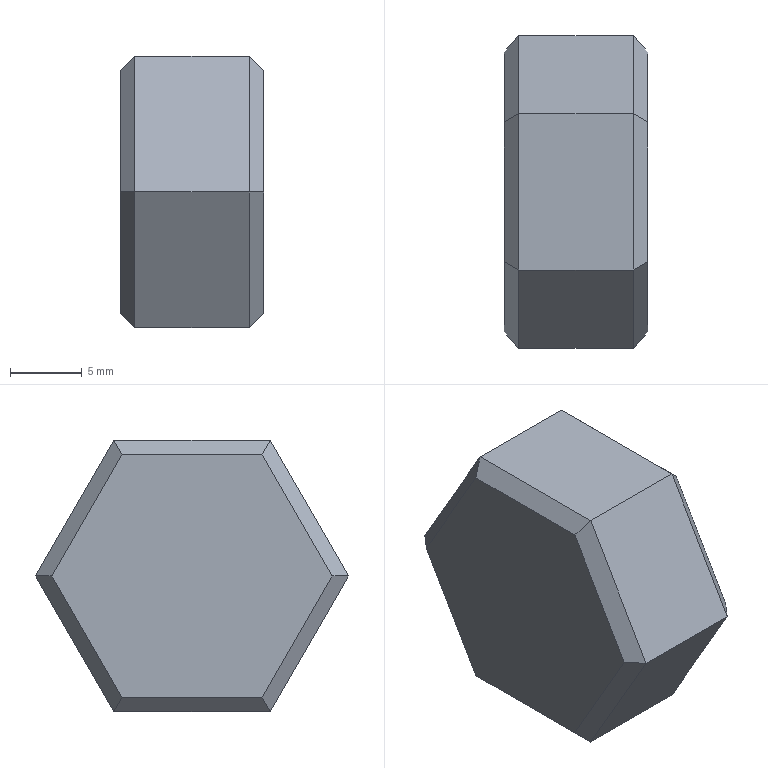Part | STEP file | Tube feed_id798_x_t | 1 solid | 20 faces | box 10 x 21.824 x 18.9 mm | volume 3030 mm3 | plane 20
STEP:
#1=CARTESIAN_POINT('',(0.,0.,0.));
#2=DIRECTION('',(0.,0.,1.));
#3=DIRECTION('',(1.,0.,0.));
#4=AXIS2_PLACEMENT_3D('',#1,#2,#3);
#5=CARTESIAN_POINT('',(413.,4.58,-40.45));
#6=VERTEX_POINT('',#5);
#7=CARTESIAN_POINT('',(421.,4.58,-40.45));
#8=VERTEX_POINT('',#7);
#9=CARTESIAN_POINT('',(412.,4.58,-40.45));
#10=DIRECTION('',(1.,0.,0.));
#11=VECTOR('',#10,1.);
#12=LINE('',#9,#11);
#13=CARTESIAN_POINT('',(412.,4.58,-40.45));
#14=DIRECTION('',(0.,0.866,0.5));
#15=DIRECTION('',(0.,-0.5,0.866));
#16=AXIS2_PLACEMENT_3D('',#13,#14,#15);
#17=PLANE('',#16);
#18=CARTESIAN_POINT('',(0.,0.));
#19=DIRECTION('',(0.,1.));
#20=VECTOR('',#19,1.);
#21=LINE('',#18,#20);
#22=(GEOMETRIC_REPRESENTATION_CONTEXT(2)PARAMETRIC_REPRESENTATION_CONTEXT()REPRESENTATION_CONTEXT('',''));
#23=DEFINITIONAL_REPRESENTATION('',(#21),#22);
#24=PCURVE('',#17,#23);
#25=CARTESIAN_POINT('',(412.,15.492,-40.45));
#26=DIRECTION('',(0.,0.,1.));
#27=DIRECTION('',(0.,-1.,0.));
#28=AXIS2_PLACEMENT_3D('',#25,#26,#27);
#29=PLANE('',#28);
#30=CARTESIAN_POINT('',(10.912,0.));
#31=DIRECTION('',(0.,1.));
#32=VECTOR('',#31,1.);
#33=LINE('',#30,#32);
#34=(GEOMETRIC_REPRESENTATION_CONTEXT(2)PARAMETRIC_REPRESENTATION_CONTEXT()REPRESENTATION_CONTEXT('',''));
#35=DEFINITIONAL_REPRESENTATION('',(#33),#34);
#36=PCURVE('',#29,#35);
#37=SURFACE_CURVE('',#12,(#24,#36),.PCURVE_S1.);
#38=EDGE_CURVE('',#6,#8,#37,.T.);
#39=ORIENTED_EDGE('',*,*,#38,.T.);
#40=CARTESIAN_POINT('',(421.,-0.8763,-31.));
#41=VERTEX_POINT('',#40);
#42=CARTESIAN_POINT('',(421.,4.58,-40.45));
#43=DIRECTION('',(0.,-0.5,0.866));
#44=VECTOR('',#43,1.);
#45=LINE('',#42,#44);
#46=CARTESIAN_POINT('',(0.,9.));
#47=DIRECTION('',(1.,0.));
#48=VECTOR('',#47,1.);
#49=LINE('',#46,#48);
#50=(GEOMETRIC_REPRESENTATION_CONTEXT(2)PARAMETRIC_REPRESENTATION_CONTEXT()REPRESENTATION_CONTEXT('',''));
#51=DEFINITIONAL_REPRESENTATION('',(#49),#50);
#52=PCURVE('',#17,#51);
#53=CARTESIAN_POINT('',(421.,4.58,-40.45));
#54=DIRECTION('',(-0.7071,0.6124,0.3536));
#55=DIRECTION('',(0.,-0.5,0.866));
#56=AXIS2_PLACEMENT_3D('',#53,#54,#55);
#57=PLANE('',#56);
#58=CARTESIAN_POINT('',(0.,0.));
#59=DIRECTION('',(1.,0.));
#60=VECTOR('',#59,1.);
#61=LINE('',#58,#60);
#62=(GEOMETRIC_REPRESENTATION_CONTEXT(2)PARAMETRIC_REPRESENTATION_CONTEXT()REPRESENTATION_CONTEXT('',''));
#63=DEFINITIONAL_REPRESENTATION('',(#61),#62);
#64=PCURVE('',#57,#63);
#65=SURFACE_CURVE('',#45,(#52,#64),.PCURVE_S1.);
#66=EDGE_CURVE('',#8,#41,#65,.T.);
#67=ORIENTED_EDGE('',*,*,#66,.T.);
#68=CARTESIAN_POINT('',(413.,-0.8763,-31.));
#69=VERTEX_POINT('',#68);
#70=CARTESIAN_POINT('',(412.,-0.8763,-31.));
#71=DIRECTION('',(1.,0.,0.));
#72=VECTOR('',#71,1.);
#73=LINE('',#70,#72);
#74=CARTESIAN_POINT('',(10.912,0.));
#75=DIRECTION('',(0.,1.));
#76=VECTOR('',#75,1.);
#77=LINE('',#74,#76);
#78=(GEOMETRIC_REPRESENTATION_CONTEXT(2)PARAMETRIC_REPRESENTATION_CONTEXT()REPRESENTATION_CONTEXT('',''));
#79=DEFINITIONAL_REPRESENTATION('',(#77),#78);
#80=PCURVE('',#17,#79);
#81=CARTESIAN_POINT('',(412.,-0.8763,-31.));
#82=DIRECTION('',(0.,0.866,-0.5));
#83=DIRECTION('',(0.,0.5,0.866));
#84=AXIS2_PLACEMENT_3D('',#81,#82,#83);
#85=PLANE('',#84);
#86=CARTESIAN_POINT('',(0.,0.));
#87=DIRECTION('',(0.,1.));
#88=VECTOR('',#87,1.);
#89=LINE('',#86,#88);
#90=(GEOMETRIC_REPRESENTATION_CONTEXT(2)PARAMETRIC_REPRESENTATION_CONTEXT()REPRESENTATION_CONTEXT('',''));
#91=DEFINITIONAL_REPRESENTATION('',(#89),#90);
#92=PCURVE('',#85,#91);
#93=SURFACE_CURVE('',#73,(#80,#92),.PCURVE_S1.);
#94=EDGE_CURVE('',#69,#41,#93,.T.);
#95=ORIENTED_EDGE('',*,*,#94,.F.);
#96=CARTESIAN_POINT('',(413.,4.58,-40.45));
#97=DIRECTION('',(0.,0.5,-0.866));
#98=VECTOR('',#97,1.);
#99=LINE('',#96,#98);
#100=CARTESIAN_POINT('',(0.,1.));
#101=DIRECTION('',(-1.,0.));
#102=VECTOR('',#101,1.);
#103=LINE('',#100,#102);
#104=(GEOMETRIC_REPRESENTATION_CONTEXT(2)PARAMETRIC_REPRESENTATION_CONTEXT()REPRESENTATION_CONTEXT('',''));
#105=DEFINITIONAL_REPRESENTATION('',(#103),#104);
#106=PCURVE('',#17,#105);
#107=CARTESIAN_POINT('',(412.,-13.215,-7.629));
#108=DIRECTION('',(-0.7071,-0.6124,-0.3536));
#109=DIRECTION('',(0.,0.5,-0.866));
#110=AXIS2_PLACEMENT_3D('',#107,#108,#109);
#111=PLANE('',#110);
#112=CARTESIAN_POINT('',(37.321,1.414));
#113=DIRECTION('',(1.,0.));
#114=VECTOR('',#113,1.);
#115=LINE('',#112,#114);
#116=(GEOMETRIC_REPRESENTATION_CONTEXT(2)PARAMETRIC_REPRESENTATION_CONTEXT()REPRESENTATION_CONTEXT('',''));
#117=DEFINITIONAL_REPRESENTATION('',(#115),#116);
#118=PCURVE('',#111,#117);
#119=SURFACE_CURVE('',#99,(#106,#118),.PCURVE_S1.);
#120=EDGE_CURVE('',#69,#6,#119,.T.);
#121=ORIENTED_EDGE('',*,*,#120,.T.);
#122=EDGE_LOOP('',(#39,#67,#95,#121));
#123=FACE_BOUND('',#122,.T.);
#124=ADVANCED_FACE('',(#123),#17,.F.);
#125=ORIENTED_EDGE('',*,*,#94,.T.);
#126=CARTESIAN_POINT('',(421.,4.58,-21.55));
#127=VERTEX_POINT('',#126);
#128=CARTESIAN_POINT('',(421.,-0.8763,-31.));
#129=DIRECTION('',(0.,0.5,0.866));
#130=VECTOR('',#129,1.);
#131=LINE('',#128,#130);
#132=CARTESIAN_POINT('',(0.,9.));
#133=DIRECTION('',(1.,0.));
#134=VECTOR('',#133,1.);
#135=LINE('',#132,#134);
#136=(GEOMETRIC_REPRESENTATION_CONTEXT(2)PARAMETRIC_REPRESENTATION_CONTEXT()REPRESENTATION_CONTEXT('',''));
#137=DEFINITIONAL_REPRESENTATION('',(#135),#136);
#138=PCURVE('',#85,#137);
#139=CARTESIAN_POINT('',(421.,-0.8763,-31.));
#140=DIRECTION('',(-0.7071,0.6124,-0.3536));
#141=DIRECTION('',(0.,0.5,0.866));
#142=AXIS2_PLACEMENT_3D('',#139,#140,#141);
#143=PLANE('',#142);
#144=CARTESIAN_POINT('',(0.,0.));
#145=DIRECTION('',(1.,0.));
#146=VECTOR('',#145,1.);
#147=LINE('',#144,#146);
#148=(GEOMETRIC_REPRESENTATION_CONTEXT(2)PARAMETRIC_REPRESENTATION_CONTEXT()REPRESENTATION_CONTEXT('',''));
#149=DEFINITIONAL_REPRESENTATION('',(#147),#148);
#150=PCURVE('',#143,#149);
#151=SURFACE_CURVE('',#131,(#138,#150),.PCURVE_S1.);
#152=EDGE_CURVE('',#41,#127,#151,.T.);
#153=ORIENTED_EDGE('',*,*,#152,.T.);
#154=CARTESIAN_POINT('',(413.,4.58,-21.55));
#155=VERTEX_POINT('',#154);
#156=CARTESIAN_POINT('',(412.,4.58,-21.55));
#157=DIRECTION('',(1.,0.,0.));
#158=VECTOR('',#157,1.);
#159=LINE('',#156,#158);
#160=CARTESIAN_POINT('',(10.912,0.));
#161=DIRECTION('',(0.,1.));
#162=VECTOR('',#161,1.);
#163=LINE('',#160,#162);
#164=(GEOMETRIC_REPRESENTATION_CONTEXT(2)PARAMETRIC_REPRESENTATION_CONTEXT()REPRESENTATION_CONTEXT('',''));
#165=DEFINITIONAL_REPRESENTATION('',(#163),#164);
#166=PCURVE('',#85,#165);
#167=CARTESIAN_POINT('',(412.,4.58,-21.55));
#168=DIRECTION('',(0.,0.,-1.));
#169=DIRECTION('',(-1.,0.,0.));
#170=AXIS2_PLACEMENT_3D('',#167,#168,#169);
#171=PLANE('',#170);
#172=CARTESIAN_POINT('',(0.,0.));
#173=DIRECTION('',(-1.,0.));
#174=VECTOR('',#173,1.);
#175=LINE('',#172,#174);
#176=(GEOMETRIC_REPRESENTATION_CONTEXT(2)PARAMETRIC_REPRESENTATION_CONTEXT()REPRESENTATION_CONTEXT('',''));
#177=DEFINITIONAL_REPRESENTATION('',(#175),#176);
#178=PCURVE('',#171,#177);
#179=SURFACE_CURVE('',#159,(#166,#178),.PCURVE_S1.);
#180=EDGE_CURVE('',#155,#127,#179,.T.);
#181=ORIENTED_EDGE('',*,*,#180,.F.);
#182=CARTESIAN_POINT('',(413.,-0.8763,-31.));
#183=DIRECTION('',(0.,-0.5,-0.866));
#184=VECTOR('',#183,1.);
#185=LINE('',#182,#184);
#186=CARTESIAN_POINT('',(0.,1.));
#187=DIRECTION('',(-1.,0.));
#188=VECTOR('',#187,1.);
#189=LINE('',#186,#188);
#190=(GEOMETRIC_REPRESENTATION_CONTEXT(2)PARAMETRIC_REPRESENTATION_CONTEXT()REPRESENTATION_CONTEXT('',''));
#191=DEFINITIONAL_REPRESENTATION('',(#189),#190);
#192=PCURVE('',#85,#191);
#193=CARTESIAN_POINT('',(412.,13.632,-7.871));
#194=DIRECTION('',(-0.7071,-0.6124,0.3536));
#195=DIRECTION('',(0.,-0.5,-0.866));
#196=AXIS2_PLACEMENT_3D('',#193,#194,#195);
#197=PLANE('',#196);
#198=CARTESIAN_POINT('',(27.285,1.414));
#199=DIRECTION('',(1.,0.));
#200=VECTOR('',#199,1.);
#201=LINE('',#198,#200);
#202=(GEOMETRIC_REPRESENTATION_CONTEXT(2)PARAMETRIC_REPRESENTATION_CONTEXT()REPRESENTATION_CONTEXT('',''));
#203=DEFINITIONAL_REPRESENTATION('',(#201),#202);
#204=PCURVE('',#197,#203);
#205=SURFACE_CURVE('',#185,(#192,#204),.PCURVE_S1.);
#206=EDGE_CURVE('',#155,#69,#205,.T.);
#207=ORIENTED_EDGE('',*,*,#206,.T.);
#208=EDGE_LOOP('',(#125,#153,#181,#207));
#209=FACE_BOUND('',#208,.T.);
#210=ADVANCED_FACE('',(#209),#85,.F.);
#211=ORIENTED_EDGE('',*,*,#180,.T.);
#212=CARTESIAN_POINT('',(421.,15.492,-21.55));
#213=VERTEX_POINT('',#212);
#214=CARTESIAN_POINT('',(421.,4.58,-21.55));
#215=DIRECTION('',(0.,1.,0.));
#216=VECTOR('',#215,1.);
#217=LINE('',#214,#216);
#218=CARTESIAN_POINT('',(-9.,0.));
#219=DIRECTION('',(0.,1.));
#220=VECTOR('',#219,1.);
#221=LINE('',#218,#220);
#222=(GEOMETRIC_REPRESENTATION_CONTEXT(2)PARAMETRIC_REPRESENTATION_CONTEXT()REPRESENTATION_CONTEXT('',''));
#223=DEFINITIONAL_REPRESENTATION('',(#221),#222);
#224=PCURVE('',#171,#223);
#225=CARTESIAN_POINT('',(421.,4.58,-21.55));
#226=DIRECTION('',(-0.7071,0.,-0.7071));
#227=DIRECTION('',(0.,1.,0.));
#228=AXIS2_PLACEMENT_3D('',#225,#226,#227);
#229=PLANE('',#228);
#230=CARTESIAN_POINT('',(0.,0.));
#231=DIRECTION('',(1.,0.));
#232=VECTOR('',#231,1.);
#233=LINE('',#230,#232);
#234=(GEOMETRIC_REPRESENTATION_CONTEXT(2)PARAMETRIC_REPRESENTATION_CONTEXT()REPRESENTATION_CONTEXT('',''));
#235=DEFINITIONAL_REPRESENTATION('',(#233),#234);
#236=PCURVE('',#229,#235);
#237=SURFACE_CURVE('',#217,(#224,#236),.PCURVE_S1.);
#238=EDGE_CURVE('',#127,#213,#237,.T.);
#239=ORIENTED_EDGE('',*,*,#238,.T.);
#240=CARTESIAN_POINT('',(413.,15.492,-21.55));
#241=VERTEX_POINT('',#240);
#242=CARTESIAN_POINT('',(412.,15.492,-21.55));
#243=DIRECTION('',(1.,0.,0.));
#244=VECTOR('',#243,1.);
#245=LINE('',#242,#244);
#246=CARTESIAN_POINT('',(0.,10.912));
#247=DIRECTION('',(-1.,0.));
#248=VECTOR('',#247,1.);
#249=LINE('',#246,#248);
#250=(GEOMETRIC_REPRESENTATION_CONTEXT(2)PARAMETRIC_REPRESENTATION_CONTEXT()REPRESENTATION_CONTEXT('',''));
#251=DEFINITIONAL_REPRESENTATION('',(#249),#250);
#252=PCURVE('',#171,#251);
#253=CARTESIAN_POINT('',(412.,15.492,-21.55));
#254=DIRECTION('',(0.,-0.866,-0.5));
#255=DIRECTION('',(0.,0.5,-0.866));
#256=AXIS2_PLACEMENT_3D('',#253,#254,#255);
#257=PLANE('',#256);
#258=CARTESIAN_POINT('',(0.,0.));
#259=DIRECTION('',(0.,1.));
#260=VECTOR('',#259,1.);
#261=LINE('',#258,#260);
#262=(GEOMETRIC_REPRESENTATION_CONTEXT(2)PARAMETRIC_REPRESENTATION_CONTEXT()REPRESENTATION_CONTEXT('',''));
#263=DEFINITIONAL_REPRESENTATION('',(#261),#262);
#264=PCURVE('',#257,#263);
#265=SURFACE_CURVE('',#245,(#252,#264),.PCURVE_S1.);
#266=EDGE_CURVE('',#241,#213,#265,.T.);
#267=ORIENTED_EDGE('',*,*,#266,.F.);
#268=CARTESIAN_POINT('',(413.,4.58,-21.55));
#269=DIRECTION('',(0.,-1.,0.));
#270=VECTOR('',#269,1.);
#271=LINE('',#268,#270);
#272=CARTESIAN_POINT('',(-1.,0.));
#273=DIRECTION('',(0.,-1.));
#274=VECTOR('',#273,1.);
#275=LINE('',#272,#274);
#276=(GEOMETRIC_REPRESENTATION_CONTEXT(2)PARAMETRIC_REPRESENTATION_CONTEXT()REPRESENTATION_CONTEXT('',''));
#277=DEFINITIONAL_REPRESENTATION('',(#275),#276);
#278=PCURVE('',#171,#277);
#279=CARTESIAN_POINT('',(412.,0.,-22.55));
#280=DIRECTION('',(-0.7071,0.,0.7071));
#281=DIRECTION('',(0.,-1.,0.));
#282=AXIS2_PLACEMENT_3D('',#279,#280,#281);
#283=PLANE('',#282);
#284=CARTESIAN_POINT('',(-4.58,1.414));
#285=DIRECTION('',(1.,0.));
#286=VECTOR('',#285,1.);
#287=LINE('',#284,#286);
#288=(GEOMETRIC_REPRESENTATION_CONTEXT(2)PARAMETRIC_REPRESENTATION_CONTEXT()REPRESENTATION_CONTEXT('',''));
#289=DEFINITIONAL_REPRESENTATION('',(#287),#288);
#290=PCURVE('',#283,#289);
#291=SURFACE_CURVE('',#271,(#278,#290),.PCURVE_S1.);
#292=EDGE_CURVE('',#241,#155,#291,.T.);
#293=ORIENTED_EDGE('',*,*,#292,.T.);
#294=EDGE_LOOP('',(#211,#239,#267,#293));
#295=FACE_BOUND('',#294,.T.);
#296=ADVANCED_FACE('',(#295),#171,.F.);
#297=ORIENTED_EDGE('',*,*,#266,.T.);
#298=CARTESIAN_POINT('',(421.,20.948,-31.));
#299=VERTEX_POINT('',#298);
#300=CARTESIAN_POINT('',(421.,15.492,-21.55));
#301=DIRECTION('',(0.,0.5,-0.866));
#302=VECTOR('',#301,1.);
#303=LINE('',#300,#302);
#304=CARTESIAN_POINT('',(0.,9.));
#305=DIRECTION('',(1.,0.));
#306=VECTOR('',#305,1.);
#307=LINE('',#304,#306);
#308=(GEOMETRIC_REPRESENTATION_CONTEXT(2)PARAMETRIC_REPRESENTATION_CONTEXT()REPRESENTATION_CONTEXT('',''));
#309=DEFINITIONAL_REPRESENTATION('',(#307),#308);
#310=PCURVE('',#257,#309);
#311=CARTESIAN_POINT('',(421.,15.492,-21.55));
#312=DIRECTION('',(-0.7071,-0.6124,-0.3536));
#313=DIRECTION('',(0.,0.5,-0.866));
#314=AXIS2_PLACEMENT_3D('',#311,#312,#313);
#315=PLANE('',#314);
#316=CARTESIAN_POINT('',(0.,0.));
#317=DIRECTION('',(1.,0.));
#318=VECTOR('',#317,1.);
#319=LINE('',#316,#318);
#320=(GEOMETRIC_REPRESENTATION_CONTEXT(2)PARAMETRIC_REPRESENTATION_CONTEXT()REPRESENTATION_CONTEXT('',''));
#321=DEFINITIONAL_REPRESENTATION('',(#319),#320);
#322=PCURVE('',#315,#321);
#323=SURFACE_CURVE('',#303,(#310,#322),.PCURVE_S1.);
#324=EDGE_CURVE('',#213,#299,#323,.T.);
#325=ORIENTED_EDGE('',*,*,#324,.T.);
#326=CARTESIAN_POINT('',(413.,20.948,-31.));
#327=VERTEX_POINT('',#326);
#328=CARTESIAN_POINT('',(412.,20.948,-31.));
#329=DIRECTION('',(1.,0.,0.));
#330=VECTOR('',#329,1.);
#331=LINE('',#328,#330);
#332=CARTESIAN_POINT('',(10.912,0.));
#333=DIRECTION('',(0.,1.));
#334=VECTOR('',#333,1.);
#335=LINE('',#332,#334);
#336=(GEOMETRIC_REPRESENTATION_CONTEXT(2)PARAMETRIC_REPRESENTATION_CONTEXT()REPRESENTATION_CONTEXT('',''));
#337=DEFINITIONAL_REPRESENTATION('',(#335),#336);
#338=PCURVE('',#257,#337);
#339=CARTESIAN_POINT('',(412.,20.948,-31.));
#340=DIRECTION('',(0.,-0.866,0.5));
#341=DIRECTION('',(0.,-0.5,-0.866));
#342=AXIS2_PLACEMENT_3D('',#339,#340,#341);
#343=PLANE('',#342);
#344=CARTESIAN_POINT('',(0.,0.));
#345=DIRECTION('',(0.,1.));
#346=VECTOR('',#345,1.);
#347=LINE('',#344,#346);
#348=(GEOMETRIC_REPRESENTATION_CONTEXT(2)PARAMETRIC_REPRESENTATION_CONTEXT()REPRESENTATION_CONTEXT('',''));
#349=DEFINITIONAL_REPRESENTATION('',(#347),#348);
#350=PCURVE('',#343,#349);
#351=SURFACE_CURVE('',#331,(#338,#350),.PCURVE_S1.);
#352=EDGE_CURVE('',#327,#299,#351,.T.);
#353=ORIENTED_EDGE('',*,*,#352,.F.);
#354=CARTESIAN_POINT('',(413.,15.492,-21.55));
#355=DIRECTION('',(0.,-0.5,0.866));
#356=VECTOR('',#355,1.);
#357=LINE('',#354,#356);
#358=CARTESIAN_POINT('',(0.,1.));
#359=DIRECTION('',(-1.,0.));
#360=VECTOR('',#359,1.);
#361=LINE('',#358,#360);
#362=(GEOMETRIC_REPRESENTATION_CONTEXT(2)PARAMETRIC_REPRESENTATION_CONTEXT()REPRESENTATION_CONTEXT('',''));
#363=DEFINITIONAL_REPRESENTATION('',(#361),#362);
#364=PCURVE('',#257,#363);
#365=CARTESIAN_POINT('',(412.,1.421,0.8206));
#366=DIRECTION('',(-0.7071,0.6124,0.3536));
#367=DIRECTION('',(0.,-0.5,0.866));
#368=AXIS2_PLACEMENT_3D('',#365,#366,#367);
#369=PLANE('',#368);
#370=CARTESIAN_POINT('',(-26.409,1.414));
#371=DIRECTION('',(1.,0.));
#372=VECTOR('',#371,1.);
#373=LINE('',#370,#372);
#374=(GEOMETRIC_REPRESENTATION_CONTEXT(2)PARAMETRIC_REPRESENTATION_CONTEXT()REPRESENTATION_CONTEXT('',''));
#375=DEFINITIONAL_REPRESENTATION('',(#373),#374);
#376=PCURVE('',#369,#375);
#377=SURFACE_CURVE('',#357,(#364,#376),.PCURVE_S1.);
#378=EDGE_CURVE('',#327,#241,#377,.T.);
#379=ORIENTED_EDGE('',*,*,#378,.T.);
#380=EDGE_LOOP('',(#297,#325,#353,#379));
#381=FACE_BOUND('',#380,.T.);
#382=ADVANCED_FACE('',(#381),#257,.F.);
#383=ORIENTED_EDGE('',*,*,#352,.T.);
#384=CARTESIAN_POINT('',(421.,15.492,-40.45));
#385=VERTEX_POINT('',#384);
#386=CARTESIAN_POINT('',(421.,20.948,-31.));
#387=DIRECTION('',(0.,-0.5,-0.866));
#388=VECTOR('',#387,1.);
#389=LINE('',#386,#388);
#390=CARTESIAN_POINT('',(0.,9.));
#391=DIRECTION('',(1.,0.));
#392=VECTOR('',#391,1.);
#393=LINE('',#390,#392);
#394=(GEOMETRIC_REPRESENTATION_CONTEXT(2)PARAMETRIC_REPRESENTATION_CONTEXT()REPRESENTATION_CONTEXT('',''));
#395=DEFINITIONAL_REPRESENTATION('',(#393),#394);
#396=PCURVE('',#343,#395);
#397=CARTESIAN_POINT('',(421.,20.948,-31.));
#398=DIRECTION('',(-0.7071,-0.6124,0.3536));
#399=DIRECTION('',(0.,-0.5,-0.866));
#400=AXIS2_PLACEMENT_3D('',#397,#398,#399);
#401=PLANE('',#400);
#402=CARTESIAN_POINT('',(0.,0.));
#403=DIRECTION('',(1.,0.));
#404=VECTOR('',#403,1.);
#405=LINE('',#402,#404);
#406=(GEOMETRIC_REPRESENTATION_CONTEXT(2)PARAMETRIC_REPRESENTATION_CONTEXT()REPRESENTATION_CONTEXT('',''));
#407=DEFINITIONAL_REPRESENTATION('',(#405),#406);
#408=PCURVE('',#401,#407);
#409=SURFACE_CURVE('',#389,(#396,#408),.PCURVE_S1.);
#410=EDGE_CURVE('',#299,#385,#409,.T.);
#411=ORIENTED_EDGE('',*,*,#410,.T.);
#412=CARTESIAN_POINT('',(413.,15.492,-40.45));
#413=VERTEX_POINT('',#412);
#414=CARTESIAN_POINT('',(412.,15.492,-40.45));
#415=DIRECTION('',(1.,0.,0.));
#416=VECTOR('',#415,1.);
#417=LINE('',#414,#416);
#418=CARTESIAN_POINT('',(10.912,0.));
#419=DIRECTION('',(0.,1.));
#420=VECTOR('',#419,1.);
#421=LINE('',#418,#420);
#422=(GEOMETRIC_REPRESENTATION_CONTEXT(2)PARAMETRIC_REPRESENTATION_CONTEXT()REPRESENTATION_CONTEXT('',''));
#423=DEFINITIONAL_REPRESENTATION('',(#421),#422);
#424=PCURVE('',#343,#423);
#425=CARTESIAN_POINT('',(0.,0.));
#426=DIRECTION('',(0.,1.));
#427=VECTOR('',#426,1.);
#428=LINE('',#425,#427);
#429=(GEOMETRIC_REPRESENTATION_CONTEXT(2)PARAMETRIC_REPRESENTATION_CONTEXT()REPRESENTATION_CONTEXT('',''));
#430=DEFINITIONAL_REPRESENTATION('',(#428),#429);
#431=PCURVE('',#29,#430);
#432=SURFACE_CURVE('',#417,(#424,#431),.PCURVE_S1.);
#433=EDGE_CURVE('',#413,#385,#432,.T.);
#434=ORIENTED_EDGE('',*,*,#433,.F.);
#435=CARTESIAN_POINT('',(413.,20.948,-31.));
#436=DIRECTION('',(0.,0.5,0.866));
#437=VECTOR('',#436,1.);
#438=LINE('',#435,#437);
#439=CARTESIAN_POINT('',(0.,1.));
#440=DIRECTION('',(-1.,0.));
#441=VECTOR('',#440,1.);
#442=LINE('',#439,#441);
#443=(GEOMETRIC_REPRESENTATION_CONTEXT(2)PARAMETRIC_REPRESENTATION_CONTEXT()REPRESENTATION_CONTEXT('',''));
#444=DEFINITIONAL_REPRESENTATION('',(#442),#443);
#445=PCURVE('',#343,#444);
#446=CARTESIAN_POINT('',(412.,28.268,-16.321));
#447=DIRECTION('',(-0.7071,0.6124,-0.3536));
#448=DIRECTION('',(0.,0.5,0.866));
#449=AXIS2_PLACEMENT_3D('',#446,#447,#448);
#450=PLANE('',#449);
#451=CARTESIAN_POINT('',(-16.373,1.414));
#452=DIRECTION('',(1.,0.));
#453=VECTOR('',#452,1.);
#454=LINE('',#451,#453);
#455=(GEOMETRIC_REPRESENTATION_CONTEXT(2)PARAMETRIC_REPRESENTATION_CONTEXT()REPRESENTATION_CONTEXT('',''));
#456=DEFINITIONAL_REPRESENTATION('',(#454),#455);
#457=PCURVE('',#450,#456);
#458=SURFACE_CURVE('',#438,(#445,#457),.PCURVE_S1.);
#459=EDGE_CURVE('',#413,#327,#458,.T.);
#460=ORIENTED_EDGE('',*,*,#459,.T.);
#461=EDGE_LOOP('',(#383,#411,#434,#460));
#462=FACE_BOUND('',#461,.T.);
#463=ADVANCED_FACE('',(#462),#343,.F.);
#464=ORIENTED_EDGE('',*,*,#433,.T.);
#465=CARTESIAN_POINT('',(421.,15.492,-40.45));
#466=DIRECTION('',(0.,-1.,0.));
#467=VECTOR('',#466,1.);
#468=LINE('',#465,#467);
#469=CARTESIAN_POINT('',(0.,9.));
#470=DIRECTION('',(1.,0.));
#471=VECTOR('',#470,1.);
#472=LINE('',#469,#471);
#473=(GEOMETRIC_REPRESENTATION_CONTEXT(2)PARAMETRIC_REPRESENTATION_CONTEXT()REPRESENTATION_CONTEXT('',''));
#474=DEFINITIONAL_REPRESENTATION('',(#472),#473);
#475=PCURVE('',#29,#474);
#476=CARTESIAN_POINT('',(421.,15.492,-40.45));
#477=DIRECTION('',(-0.7071,0.,0.7071));
#478=DIRECTION('',(0.,-1.,0.));
#479=AXIS2_PLACEMENT_3D('',#476,#477,#478);
#480=PLANE('',#479);
#481=CARTESIAN_POINT('',(0.,0.));
#482=DIRECTION('',(1.,0.));
#483=VECTOR('',#482,1.);
#484=LINE('',#481,#483);
#485=(GEOMETRIC_REPRESENTATION_CONTEXT(2)PARAMETRIC_REPRESENTATION_CONTEXT()REPRESENTATION_CONTEXT('',''));
#486=DEFINITIONAL_REPRESENTATION('',(#484),#485);
#487=PCURVE('',#480,#486);
#488=SURFACE_CURVE('',#468,(#475,#487),.PCURVE_S1.);
#489=EDGE_CURVE('',#385,#8,#488,.T.);
#490=ORIENTED_EDGE('',*,*,#489,.T.);
#491=ORIENTED_EDGE('',*,*,#38,.F.);
#492=CARTESIAN_POINT('',(413.,15.492,-40.45));
#493=DIRECTION('',(0.,1.,0.));
#494=VECTOR('',#493,1.);
#495=LINE('',#492,#494);
#496=CARTESIAN_POINT('',(0.,1.));
#497=DIRECTION('',(-1.,0.));
#498=VECTOR('',#497,1.);
#499=LINE('',#496,#498);
#500=(GEOMETRIC_REPRESENTATION_CONTEXT(2)PARAMETRIC_REPRESENTATION_CONTEXT()REPRESENTATION_CONTEXT('',''));
#501=DEFINITIONAL_REPRESENTATION('',(#499),#500);
#502=PCURVE('',#29,#501);
#503=CARTESIAN_POINT('',(412.,0.,-39.45));
#504=DIRECTION('',(-0.7071,0.,-0.7071));
#505=DIRECTION('',(0.,1.,0.));
#506=AXIS2_PLACEMENT_3D('',#503,#504,#505);
#507=PLANE('',#506);
#508=CARTESIAN_POINT('',(15.492,1.414));
#509=DIRECTION('',(1.,0.));
#510=VECTOR('',#509,1.);
#511=LINE('',#508,#510);
#512=(GEOMETRIC_REPRESENTATION_CONTEXT(2)PARAMETRIC_REPRESENTATION_CONTEXT()REPRESENTATION_CONTEXT('',''));
#513=DEFINITIONAL_REPRESENTATION('',(#511),#512);
#514=PCURVE('',#507,#513);
#515=SURFACE_CURVE('',#495,(#502,#514),.PCURVE_S1.);
#516=EDGE_CURVE('',#6,#413,#515,.T.);
#517=ORIENTED_EDGE('',*,*,#516,.T.);
#518=EDGE_LOOP('',(#464,#490,#491,#517));
#519=FACE_BOUND('',#518,.T.);
#520=ADVANCED_FACE('',(#519),#29,.F.);
#521=CARTESIAN_POINT('',(412.,14.914,-39.45));
#522=VERTEX_POINT('',#521);
#523=CARTESIAN_POINT('',(412.,5.157,-39.45));
#524=VERTEX_POINT('',#523);
#525=CARTESIAN_POINT('',(412.,4.58,-39.45));
#526=DIRECTION('',(0.,-1.,0.));
#527=VECTOR('',#526,1.);
#528=LINE('',#525,#527);
#529=CARTESIAN_POINT('',(412.,0.,0.));
#530=DIRECTION('',(-1.,0.,0.));
#531=DIRECTION('',(0.,0.,1.));
#532=AXIS2_PLACEMENT_3D('',#529,#530,#531);
#533=PLANE('',#532);
#534=CARTESIAN_POINT('',(-39.45,4.58));
#535=DIRECTION('',(0.,-1.));
#536=VECTOR('',#535,1.);
#537=LINE('',#534,#536);
#538=(GEOMETRIC_REPRESENTATION_CONTEXT(2)PARAMETRIC_REPRESENTATION_CONTEXT()REPRESENTATION_CONTEXT('',''));
#539=DEFINITIONAL_REPRESENTATION('',(#537),#538);
#540=PCURVE('',#533,#539);
#541=CARTESIAN_POINT('',(4.58,0.));
#542=DIRECTION('',(-1.,0.));
#543=VECTOR('',#542,1.);
#544=LINE('',#541,#543);
#545=(GEOMETRIC_REPRESENTATION_CONTEXT(2)PARAMETRIC_REPRESENTATION_CONTEXT()REPRESENTATION_CONTEXT('',''));
#546=DEFINITIONAL_REPRESENTATION('',(#544),#545);
#547=PCURVE('',#507,#546);
#548=SURFACE_CURVE('',#528,(#540,#547),.PCURVE_S1.);
#549=EDGE_CURVE('',#522,#524,#548,.T.);
#550=ORIENTED_EDGE('',*,*,#549,.T.);
#551=CARTESIAN_POINT('',(412.,0.2784,-31.));
#552=VERTEX_POINT('',#551);
#553=CARTESIAN_POINT('',(412.,-0.01026,-30.5));
#554=DIRECTION('',(0.,-0.5,0.866));
#555=VECTOR('',#554,1.);
#556=LINE('',#553,#555);
#557=CARTESIAN_POINT('',(-30.5,-0.01026));
#558=DIRECTION('',(0.866,-0.5));
#559=VECTOR('',#558,1.);
#560=LINE('',#557,#559);
#561=(GEOMETRIC_REPRESENTATION_CONTEXT(2)PARAMETRIC_REPRESENTATION_CONTEXT()REPRESENTATION_CONTEXT('',''));
#562=DEFINITIONAL_REPRESENTATION('',(#560),#561);
#563=PCURVE('',#533,#562);
#564=CARTESIAN_POINT('',(26.409,0.));
#565=DIRECTION('',(-1.,0.));
#566=VECTOR('',#565,1.);
#567=LINE('',#564,#566);
#568=(GEOMETRIC_REPRESENTATION_CONTEXT(2)PARAMETRIC_REPRESENTATION_CONTEXT()REPRESENTATION_CONTEXT('',''));
#569=DEFINITIONAL_REPRESENTATION('',(#567),#568);
#570=PCURVE('',#111,#569);
#571=SURFACE_CURVE('',#556,(#563,#570),.PCURVE_S1.);
#572=EDGE_CURVE('',#524,#552,#571,.T.);
#573=ORIENTED_EDGE('',*,*,#572,.T.);
#574=CARTESIAN_POINT('',(412.,5.157,-22.55));
#575=VERTEX_POINT('',#574);
#576=CARTESIAN_POINT('',(412.,5.446,-22.05));
#577=DIRECTION('',(0.,0.5,0.866));
#578=VECTOR('',#577,1.);
#579=LINE('',#576,#578);
#580=CARTESIAN_POINT('',(-22.05,5.446));
#581=DIRECTION('',(0.866,0.5));
#582=VECTOR('',#581,1.);
#583=LINE('',#580,#582);
#584=(GEOMETRIC_REPRESENTATION_CONTEXT(2)PARAMETRIC_REPRESENTATION_CONTEXT()REPRESENTATION_CONTEXT('',''));
#585=DEFINITIONAL_REPRESENTATION('',(#583),#584);
#586=PCURVE('',#533,#585);
#587=CARTESIAN_POINT('',(16.373,0.));
#588=DIRECTION('',(-1.,0.));
#589=VECTOR('',#588,1.);
#590=LINE('',#587,#589);
#591=(GEOMETRIC_REPRESENTATION_CONTEXT(2)PARAMETRIC_REPRESENTATION_CONTEXT()REPRESENTATION_CONTEXT('',''));
#592=DEFINITIONAL_REPRESENTATION('',(#590),#591);
#593=PCURVE('',#197,#592);
#594=SURFACE_CURVE('',#579,(#586,#593),.PCURVE_S1.);
#595=EDGE_CURVE('',#552,#575,#594,.T.);
#596=ORIENTED_EDGE('',*,*,#595,.T.);
#597=CARTESIAN_POINT('',(412.,14.914,-22.55));
#598=VERTEX_POINT('',#597);
#599=CARTESIAN_POINT('',(412.,15.492,-22.55));
#600=DIRECTION('',(0.,1.,0.));
#601=VECTOR('',#600,1.);
#602=LINE('',#599,#601);
#603=CARTESIAN_POINT('',(-22.55,15.492));
#604=DIRECTION('',(0.,1.));
#605=VECTOR('',#604,1.);
#606=LINE('',#603,#605);
#607=(GEOMETRIC_REPRESENTATION_CONTEXT(2)PARAMETRIC_REPRESENTATION_CONTEXT()REPRESENTATION_CONTEXT('',''));
#608=DEFINITIONAL_REPRESENTATION('',(#606),#607);
#609=PCURVE('',#533,#608);
#610=CARTESIAN_POINT('',(-15.492,0.));
#611=DIRECTION('',(-1.,0.));
#612=VECTOR('',#611,1.);
#613=LINE('',#610,#612);
#614=(GEOMETRIC_REPRESENTATION_CONTEXT(2)PARAMETRIC_REPRESENTATION_CONTEXT()REPRESENTATION_CONTEXT('',''));
#615=DEFINITIONAL_REPRESENTATION('',(#613),#614);
#616=PCURVE('',#283,#615);
#617=SURFACE_CURVE('',#602,(#609,#616),.PCURVE_S1.);
#618=EDGE_CURVE('',#575,#598,#617,.T.);
#619=ORIENTED_EDGE('',*,*,#618,.T.);
#620=CARTESIAN_POINT('',(412.,19.793,-31.));
#621=VERTEX_POINT('',#620);
#622=CARTESIAN_POINT('',(412.,20.082,-31.5));
#623=DIRECTION('',(0.,0.5,-0.866));
#624=VECTOR('',#623,1.);
#625=LINE('',#622,#624);
#626=CARTESIAN_POINT('',(-31.5,20.082));
#627=DIRECTION('',(-0.866,0.5));
#628=VECTOR('',#627,1.);
#629=LINE('',#626,#628);
#630=(GEOMETRIC_REPRESENTATION_CONTEXT(2)PARAMETRIC_REPRESENTATION_CONTEXT()REPRESENTATION_CONTEXT('',''));
#631=DEFINITIONAL_REPRESENTATION('',(#629),#630);
#632=PCURVE('',#533,#631);
#633=CARTESIAN_POINT('',(-37.321,0.));
#634=DIRECTION('',(-1.,0.));
#635=VECTOR('',#634,1.);
#636=LINE('',#633,#635);
#637=(GEOMETRIC_REPRESENTATION_CONTEXT(2)PARAMETRIC_REPRESENTATION_CONTEXT()REPRESENTATION_CONTEXT('',''));
#638=DEFINITIONAL_REPRESENTATION('',(#636),#637);
#639=PCURVE('',#369,#638);
#640=SURFACE_CURVE('',#625,(#632,#639),.PCURVE_S1.);
#641=EDGE_CURVE('',#598,#621,#640,.T.);
#642=ORIENTED_EDGE('',*,*,#641,.T.);
#643=CARTESIAN_POINT('',(412.,14.626,-39.95));
#644=DIRECTION('',(0.,-0.5,-0.866));
#645=VECTOR('',#644,1.);
#646=LINE('',#643,#645);
#647=CARTESIAN_POINT('',(-39.95,14.626));
#648=DIRECTION('',(-0.866,-0.5));
#649=VECTOR('',#648,1.);
#650=LINE('',#647,#649);
#651=(GEOMETRIC_REPRESENTATION_CONTEXT(2)PARAMETRIC_REPRESENTATION_CONTEXT()REPRESENTATION_CONTEXT('',''));
#652=DEFINITIONAL_REPRESENTATION('',(#650),#651);
#653=PCURVE('',#533,#652);
#654=CARTESIAN_POINT('',(-27.285,0.));
#655=DIRECTION('',(-1.,0.));
#656=VECTOR('',#655,1.);
#657=LINE('',#654,#656);
#658=(GEOMETRIC_REPRESENTATION_CONTEXT(2)PARAMETRIC_REPRESENTATION_CONTEXT()REPRESENTATION_CONTEXT('',''));
#659=DEFINITIONAL_REPRESENTATION('',(#657),#658);
#660=PCURVE('',#450,#659);
#661=SURFACE_CURVE('',#646,(#653,#660),.PCURVE_S1.);
#662=EDGE_CURVE('',#621,#522,#661,.T.);
#663=ORIENTED_EDGE('',*,*,#662,.T.);
#664=EDGE_LOOP('',(#550,#573,#596,#619,#642,#663));
#665=FACE_BOUND('',#664,.T.);
#666=ADVANCED_FACE('',(#665),#533,.T.);
#667=CARTESIAN_POINT('',(422.,5.157,-22.55));
#668=VERTEX_POINT('',#667);
#669=CARTESIAN_POINT('',(422.,0.2784,-31.));
#670=VERTEX_POINT('',#669);
#671=CARTESIAN_POINT('',(422.,13.632,-7.871));
#672=DIRECTION('',(0.,-0.5,-0.866));
#673=VECTOR('',#672,1.);
#674=LINE('',#671,#673);
#675=CARTESIAN_POINT('',(422.,0.,0.));
#676=DIRECTION('',(-1.,0.,0.));
#677=DIRECTION('',(0.,0.,1.));
#678=AXIS2_PLACEMENT_3D('',#675,#676,#677);
#679=PLANE('',#678);
#680=CARTESIAN_POINT('',(-7.871,13.632));
#681=DIRECTION('',(-0.866,-0.5));
#682=VECTOR('',#681,1.);
#683=LINE('',#680,#682);
#684=(GEOMETRIC_REPRESENTATION_CONTEXT(2)PARAMETRIC_REPRESENTATION_CONTEXT()REPRESENTATION_CONTEXT('',''));
#685=DEFINITIONAL_REPRESENTATION('',(#683),#684);
#686=PCURVE('',#679,#685);
#687=CARTESIAN_POINT('',(27.285,1.414));
#688=DIRECTION('',(-1.,0.));
#689=VECTOR('',#688,1.);
#690=LINE('',#687,#689);
#691=(GEOMETRIC_REPRESENTATION_CONTEXT(2)PARAMETRIC_REPRESENTATION_CONTEXT()REPRESENTATION_CONTEXT('',''));
#692=DEFINITIONAL_REPRESENTATION('',(#690),#691);
#693=PCURVE('',#143,#692);
#694=SURFACE_CURVE('',#674,(#686,#693),.PCURVE_S1.);
#695=EDGE_CURVE('',#668,#670,#694,.T.);
#696=ORIENTED_EDGE('',*,*,#695,.T.);
#697=CARTESIAN_POINT('',(422.,5.157,-39.45));
#698=VERTEX_POINT('',#697);
#699=CARTESIAN_POINT('',(422.,-13.215,-7.629));
#700=DIRECTION('',(0.,0.5,-0.866));
#701=VECTOR('',#700,1.);
#702=LINE('',#699,#701);
#703=CARTESIAN_POINT('',(-7.629,-13.215));
#704=DIRECTION('',(-0.866,0.5));
#705=VECTOR('',#704,1.);
#706=LINE('',#703,#705);
#707=(GEOMETRIC_REPRESENTATION_CONTEXT(2)PARAMETRIC_REPRESENTATION_CONTEXT()REPRESENTATION_CONTEXT('',''));
#708=DEFINITIONAL_REPRESENTATION('',(#706),#707);
#709=PCURVE('',#679,#708);
#710=CARTESIAN_POINT('',(37.321,1.414));
#711=DIRECTION('',(-1.,0.));
#712=VECTOR('',#711,1.);
#713=LINE('',#710,#712);
#714=(GEOMETRIC_REPRESENTATION_CONTEXT(2)PARAMETRIC_REPRESENTATION_CONTEXT()REPRESENTATION_CONTEXT('',''));
#715=DEFINITIONAL_REPRESENTATION('',(#713),#714);
#716=PCURVE('',#57,#715);
#717=SURFACE_CURVE('',#702,(#709,#716),.PCURVE_S1.);
#718=EDGE_CURVE('',#670,#698,#717,.T.);
#719=ORIENTED_EDGE('',*,*,#718,.T.);
#720=CARTESIAN_POINT('',(422.,14.914,-39.45));
#721=VERTEX_POINT('',#720);
#722=CARTESIAN_POINT('',(422.,0.,-39.45));
#723=DIRECTION('',(0.,1.,0.));
#724=VECTOR('',#723,1.);
#725=LINE('',#722,#724);
#726=CARTESIAN_POINT('',(-39.45,0.));
#727=DIRECTION('',(0.,1.));
#728=VECTOR('',#727,1.);
#729=LINE('',#726,#728);
#730=(GEOMETRIC_REPRESENTATION_CONTEXT(2)PARAMETRIC_REPRESENTATION_CONTEXT()REPRESENTATION_CONTEXT('',''));
#731=DEFINITIONAL_REPRESENTATION('',(#729),#730);
#732=PCURVE('',#679,#731);
#733=CARTESIAN_POINT('',(15.492,1.414));
#734=DIRECTION('',(-1.,0.));
#735=VECTOR('',#734,1.);
#736=LINE('',#733,#735);
#737=(GEOMETRIC_REPRESENTATION_CONTEXT(2)PARAMETRIC_REPRESENTATION_CONTEXT()REPRESENTATION_CONTEXT('',''));
#738=DEFINITIONAL_REPRESENTATION('',(#736),#737);
#739=PCURVE('',#480,#738);
#740=SURFACE_CURVE('',#725,(#732,#739),.PCURVE_S1.);
#741=EDGE_CURVE('',#698,#721,#740,.T.);
#742=ORIENTED_EDGE('',*,*,#741,.T.);
#743=CARTESIAN_POINT('',(422.,19.793,-31.));
#744=VERTEX_POINT('',#743);
#745=CARTESIAN_POINT('',(422.,28.268,-16.321));
#746=DIRECTION('',(0.,0.5,0.866));
#747=VECTOR('',#746,1.);
#748=LINE('',#745,#747);
#749=CARTESIAN_POINT('',(-16.321,28.268));
#750=DIRECTION('',(0.866,0.5));
#751=VECTOR('',#750,1.);
#752=LINE('',#749,#751);
#753=(GEOMETRIC_REPRESENTATION_CONTEXT(2)PARAMETRIC_REPRESENTATION_CONTEXT()REPRESENTATION_CONTEXT('',''));
#754=DEFINITIONAL_REPRESENTATION('',(#752),#753);
#755=PCURVE('',#679,#754);
#756=CARTESIAN_POINT('',(-16.373,1.414));
#757=DIRECTION('',(-1.,0.));
#758=VECTOR('',#757,1.);
#759=LINE('',#756,#758);
#760=(GEOMETRIC_REPRESENTATION_CONTEXT(2)PARAMETRIC_REPRESENTATION_CONTEXT()REPRESENTATION_CONTEXT('',''));
#761=DEFINITIONAL_REPRESENTATION('',(#759),#760);
#762=PCURVE('',#401,#761);
#763=SURFACE_CURVE('',#748,(#755,#762),.PCURVE_S1.);
#764=EDGE_CURVE('',#721,#744,#763,.T.);
#765=ORIENTED_EDGE('',*,*,#764,.T.);
#766=CARTESIAN_POINT('',(422.,14.914,-22.55));
#767=VERTEX_POINT('',#766);
#768=CARTESIAN_POINT('',(422.,1.421,0.8206));
#769=DIRECTION('',(0.,-0.5,0.866));
#770=VECTOR('',#769,1.);
#771=LINE('',#768,#770);
#772=CARTESIAN_POINT('',(0.8206,1.421));
#773=DIRECTION('',(0.866,-0.5));
#774=VECTOR('',#773,1.);
#775=LINE('',#772,#774);
#776=(GEOMETRIC_REPRESENTATION_CONTEXT(2)PARAMETRIC_REPRESENTATION_CONTEXT()REPRESENTATION_CONTEXT('',''));
#777=DEFINITIONAL_REPRESENTATION('',(#775),#776);
#778=PCURVE('',#679,#777);
#779=CARTESIAN_POINT('',(-26.409,1.414));
#780=DIRECTION('',(-1.,0.));
#781=VECTOR('',#780,1.);
#782=LINE('',#779,#781);
#783=(GEOMETRIC_REPRESENTATION_CONTEXT(2)PARAMETRIC_REPRESENTATION_CONTEXT()REPRESENTATION_CONTEXT('',''));
#784=DEFINITIONAL_REPRESENTATION('',(#782),#783);
#785=PCURVE('',#315,#784);
#786=SURFACE_CURVE('',#771,(#778,#785),.PCURVE_S1.);
#787=EDGE_CURVE('',#744,#767,#786,.T.);
#788=ORIENTED_EDGE('',*,*,#787,.T.);
#789=CARTESIAN_POINT('',(422.,0.,-22.55));
#790=DIRECTION('',(0.,-1.,0.));
#791=VECTOR('',#790,1.);
#792=LINE('',#789,#791);
#793=CARTESIAN_POINT('',(-22.55,0.));
#794=DIRECTION('',(0.,-1.));
#795=VECTOR('',#794,1.);
#796=LINE('',#793,#795);
#797=(GEOMETRIC_REPRESENTATION_CONTEXT(2)PARAMETRIC_REPRESENTATION_CONTEXT()REPRESENTATION_CONTEXT('',''));
#798=DEFINITIONAL_REPRESENTATION('',(#796),#797);
#799=PCURVE('',#679,#798);
#800=CARTESIAN_POINT('',(-4.58,1.414));
#801=DIRECTION('',(-1.,0.));
#802=VECTOR('',#801,1.);
#803=LINE('',#800,#802);
#804=(GEOMETRIC_REPRESENTATION_CONTEXT(2)PARAMETRIC_REPRESENTATION_CONTEXT()REPRESENTATION_CONTEXT('',''));
#805=DEFINITIONAL_REPRESENTATION('',(#803),#804);
#806=PCURVE('',#229,#805);
#807=SURFACE_CURVE('',#792,(#799,#806),.PCURVE_S1.);
#808=EDGE_CURVE('',#767,#668,#807,.T.);
#809=ORIENTED_EDGE('',*,*,#808,.T.);
#810=EDGE_LOOP('',(#696,#719,#742,#765,#788,#809));
#811=FACE_BOUND('',#810,.T.);
#812=ADVANCED_FACE('',(#811),#679,.F.);
#813=CARTESIAN_POINT('',(421.,15.492,-21.55));
#814=DIRECTION('',(-0.6547,0.378,0.6547));
#815=VECTOR('',#814,1.);
#816=LINE('',#813,#815);
#817=CARTESIAN_POINT('',(0.,0.));
#818=DIRECTION('',(-0.378,-0.9258));
#819=VECTOR('',#818,1.);
#820=LINE('',#817,#819);
#821=(GEOMETRIC_REPRESENTATION_CONTEXT(2)PARAMETRIC_REPRESENTATION_CONTEXT()REPRESENTATION_CONTEXT('',''));
#822=DEFINITIONAL_REPRESENTATION('',(#820),#821);
#823=PCURVE('',#315,#822);
#824=CARTESIAN_POINT('',(10.912,0.));
#825=DIRECTION('',(0.378,-0.9258));
#826=VECTOR('',#825,1.);
#827=LINE('',#824,#826);
#828=(GEOMETRIC_REPRESENTATION_CONTEXT(2)PARAMETRIC_REPRESENTATION_CONTEXT()REPRESENTATION_CONTEXT('',''));
#829=DEFINITIONAL_REPRESENTATION('',(#827),#828);
#830=PCURVE('',#229,#829);
#831=SURFACE_CURVE('',#816,(#823,#830),.PCURVE_S1.);
#832=EDGE_CURVE('',#767,#213,#831,.T.);
#833=ORIENTED_EDGE('',*,*,#832,.F.);
#834=ORIENTED_EDGE('',*,*,#787,.F.);
#835=CARTESIAN_POINT('',(421.,20.948,-31.));
#836=DIRECTION('',(0.6547,-0.7559,0.));
#837=VECTOR('',#836,1.);
#838=LINE('',#835,#837);
#839=CARTESIAN_POINT('',(10.912,0.));
#840=DIRECTION('',(-0.378,0.9258));
#841=VECTOR('',#840,1.);
#842=LINE('',#839,#841);
#843=(GEOMETRIC_REPRESENTATION_CONTEXT(2)PARAMETRIC_REPRESENTATION_CONTEXT()REPRESENTATION_CONTEXT('',''));
#844=DEFINITIONAL_REPRESENTATION('',(#842),#843);
#845=PCURVE('',#315,#844);
#846=CARTESIAN_POINT('',(0.,0.));
#847=DIRECTION('',(0.378,0.9258));
#848=VECTOR('',#847,1.);
#849=LINE('',#846,#848);
#850=(GEOMETRIC_REPRESENTATION_CONTEXT(2)PARAMETRIC_REPRESENTATION_CONTEXT()REPRESENTATION_CONTEXT('',''));
#851=DEFINITIONAL_REPRESENTATION('',(#849),#850);
#852=PCURVE('',#401,#851);
#853=SURFACE_CURVE('',#838,(#845,#852),.PCURVE_S1.);
#854=EDGE_CURVE('',#299,#744,#853,.T.);
#855=ORIENTED_EDGE('',*,*,#854,.F.);
#856=ORIENTED_EDGE('',*,*,#324,.F.);
#857=EDGE_LOOP('',(#833,#834,#855,#856));
#858=FACE_BOUND('',#857,.T.);
#859=ADVANCED_FACE('',(#858),#315,.F.);
#860=ORIENTED_EDGE('',*,*,#854,.T.);
#861=ORIENTED_EDGE('',*,*,#764,.F.);
#862=CARTESIAN_POINT('',(421.,15.492,-40.45));
#863=DIRECTION('',(0.6547,-0.378,0.6547));
#864=VECTOR('',#863,1.);
#865=LINE('',#862,#864);
#866=CARTESIAN_POINT('',(10.912,0.));
#867=DIRECTION('',(-0.378,0.9258));
#868=VECTOR('',#867,1.);
#869=LINE('',#866,#868);
#870=(GEOMETRIC_REPRESENTATION_CONTEXT(2)PARAMETRIC_REPRESENTATION_CONTEXT()REPRESENTATION_CONTEXT('',''));
#871=DEFINITIONAL_REPRESENTATION('',(#869),#870);
#872=PCURVE('',#401,#871);
#873=CARTESIAN_POINT('',(0.,0.));
#874=DIRECTION('',(0.378,0.9258));
#875=VECTOR('',#874,1.);
#876=LINE('',#873,#875);
#877=(GEOMETRIC_REPRESENTATION_CONTEXT(2)PARAMETRIC_REPRESENTATION_CONTEXT()REPRESENTATION_CONTEXT('',''));
#878=DEFINITIONAL_REPRESENTATION('',(#876),#877);
#879=PCURVE('',#480,#878);
#880=SURFACE_CURVE('',#865,(#872,#879),.PCURVE_S1.);
#881=EDGE_CURVE('',#385,#721,#880,.T.);
#882=ORIENTED_EDGE('',*,*,#881,.F.);
#883=ORIENTED_EDGE('',*,*,#410,.F.);
#884=EDGE_LOOP('',(#860,#861,#882,#883));
#885=FACE_BOUND('',#884,.T.);
#886=ADVANCED_FACE('',(#885),#401,.F.);
#887=ORIENTED_EDGE('',*,*,#832,.T.);
#888=ORIENTED_EDGE('',*,*,#238,.F.);
#889=CARTESIAN_POINT('',(421.,4.58,-21.55));
#890=DIRECTION('',(-0.6547,-0.378,0.6547));
#891=VECTOR('',#890,1.);
#892=LINE('',#889,#891);
#893=CARTESIAN_POINT('',(0.,0.));
#894=DIRECTION('',(-0.378,-0.9258));
#895=VECTOR('',#894,1.);
#896=LINE('',#893,#895);
#897=(GEOMETRIC_REPRESENTATION_CONTEXT(2)PARAMETRIC_REPRESENTATION_CONTEXT()REPRESENTATION_CONTEXT('',''));
#898=DEFINITIONAL_REPRESENTATION('',(#896),#897);
#899=PCURVE('',#229,#898);
#900=CARTESIAN_POINT('',(10.912,0.));
#901=DIRECTION('',(0.378,-0.9258));
#902=VECTOR('',#901,1.);
#903=LINE('',#900,#902);
#904=(GEOMETRIC_REPRESENTATION_CONTEXT(2)PARAMETRIC_REPRESENTATION_CONTEXT()REPRESENTATION_CONTEXT('',''));
#905=DEFINITIONAL_REPRESENTATION('',(#903),#904);
#906=PCURVE('',#143,#905);
#907=SURFACE_CURVE('',#892,(#899,#906),.PCURVE_S1.);
#908=EDGE_CURVE('',#668,#127,#907,.T.);
#909=ORIENTED_EDGE('',*,*,#908,.F.);
#910=ORIENTED_EDGE('',*,*,#808,.F.);
#911=EDGE_LOOP('',(#887,#888,#909,#910));
#912=FACE_BOUND('',#911,.T.);
#913=ADVANCED_FACE('',(#912),#229,.F.);
#914=ORIENTED_EDGE('',*,*,#881,.T.);
#915=ORIENTED_EDGE('',*,*,#741,.F.);
#916=CARTESIAN_POINT('',(423.7,6.139,-37.75));
#917=DIRECTION('',(0.6547,0.378,0.6547));
#918=VECTOR('',#917,1.);
#919=LINE('',#916,#918);
#920=CARTESIAN_POINT('',(9.353,3.818));
#921=DIRECTION('',(-0.378,0.9258));
#922=VECTOR('',#921,1.);
#923=LINE('',#920,#922);
#924=(GEOMETRIC_REPRESENTATION_CONTEXT(2)PARAMETRIC_REPRESENTATION_CONTEXT()REPRESENTATION_CONTEXT('',''));
#925=DEFINITIONAL_REPRESENTATION('',(#923),#924);
#926=PCURVE('',#480,#925);
#927=CARTESIAN_POINT('',(1.559,3.818));
#928=DIRECTION('',(0.378,0.9258));
#929=VECTOR('',#928,1.);
#930=LINE('',#927,#929);
#931=(GEOMETRIC_REPRESENTATION_CONTEXT(2)PARAMETRIC_REPRESENTATION_CONTEXT()REPRESENTATION_CONTEXT('',''));
#932=DEFINITIONAL_REPRESENTATION('',(#930),#931);
#933=PCURVE('',#57,#932);
#934=SURFACE_CURVE('',#919,(#926,#933),.PCURVE_S1.);
#935=EDGE_CURVE('',#8,#698,#934,.T.);
#936=ORIENTED_EDGE('',*,*,#935,.F.);
#937=ORIENTED_EDGE('',*,*,#489,.F.);
#938=EDGE_LOOP('',(#914,#915,#936,#937));
#939=FACE_BOUND('',#938,.T.);
#940=ADVANCED_FACE('',(#939),#480,.F.);
#941=ORIENTED_EDGE('',*,*,#908,.T.);
#942=ORIENTED_EDGE('',*,*,#152,.F.);
#943=CARTESIAN_POINT('',(421.,-0.8763,-31.));
#944=DIRECTION('',(-0.6547,-0.7559,0.));
#945=VECTOR('',#944,1.);
#946=LINE('',#943,#945);
#947=CARTESIAN_POINT('',(0.,0.));
#948=DIRECTION('',(-0.378,-0.9258));
#949=VECTOR('',#948,1.);
#950=LINE('',#947,#949);
#951=(GEOMETRIC_REPRESENTATION_CONTEXT(2)PARAMETRIC_REPRESENTATION_CONTEXT()REPRESENTATION_CONTEXT('',''));
#952=DEFINITIONAL_REPRESENTATION('',(#950),#951);
#953=PCURVE('',#143,#952);
#954=CARTESIAN_POINT('',(10.912,0.));
#955=DIRECTION('',(0.378,-0.9258));
#956=VECTOR('',#955,1.);
#957=LINE('',#954,#956);
#958=(GEOMETRIC_REPRESENTATION_CONTEXT(2)PARAMETRIC_REPRESENTATION_CONTEXT()REPRESENTATION_CONTEXT('',''));
#959=DEFINITIONAL_REPRESENTATION('',(#957),#958);
#960=PCURVE('',#57,#959);
#961=SURFACE_CURVE('',#946,(#953,#960),.PCURVE_S1.);
#962=EDGE_CURVE('',#670,#41,#961,.T.);
#963=ORIENTED_EDGE('',*,*,#962,.F.);
#964=ORIENTED_EDGE('',*,*,#695,.F.);
#965=EDGE_LOOP('',(#941,#942,#963,#964));
#966=FACE_BOUND('',#965,.T.);
#967=ADVANCED_FACE('',(#966),#143,.F.);
#968=ORIENTED_EDGE('',*,*,#935,.T.);
#969=ORIENTED_EDGE('',*,*,#718,.F.);
#970=ORIENTED_EDGE('',*,*,#962,.T.);
#971=ORIENTED_EDGE('',*,*,#66,.F.);
#972=EDGE_LOOP('',(#968,#969,#970,#971));
#973=FACE_BOUND('',#972,.T.);
#974=ADVANCED_FACE('',(#973),#57,.F.);
#975=CARTESIAN_POINT('',(418.677,18.769,-15.873));
#976=DIRECTION('',(-0.6547,-0.378,-0.6547));
#977=VECTOR('',#976,1.);
#978=LINE('',#975,#977);
#979=CARTESIAN_POINT('',(-23.131,9.443));
#980=DIRECTION('',(-0.378,-0.9258));
#981=VECTOR('',#980,1.);
#982=LINE('',#979,#981);
#983=(GEOMETRIC_REPRESENTATION_CONTEXT(2)PARAMETRIC_REPRESENTATION_CONTEXT()REPRESENTATION_CONTEXT('',''));
#984=DEFINITIONAL_REPRESENTATION('',(#982),#983);
#985=PCURVE('',#369,#984);
#986=CARTESIAN_POINT('',(-18.769,9.443));
#987=DIRECTION('',(0.378,-0.9258));
#988=VECTOR('',#987,1.);
#989=LINE('',#986,#988);
#990=(GEOMETRIC_REPRESENTATION_CONTEXT(2)PARAMETRIC_REPRESENTATION_CONTEXT()REPRESENTATION_CONTEXT('',''));
#991=DEFINITIONAL_REPRESENTATION('',(#989),#990);
#992=PCURVE('',#283,#991);
#993=SURFACE_CURVE('',#978,(#985,#992),.PCURVE_S1.);
#994=EDGE_CURVE('',#241,#598,#993,.T.);
#995=ORIENTED_EDGE('',*,*,#994,.F.);
#996=ORIENTED_EDGE('',*,*,#378,.F.);
#997=CARTESIAN_POINT('',(416.194,24.636,-31.));
#998=DIRECTION('',(0.6547,0.7559,0.));
#999=VECTOR('',#998,1.);
#1000=LINE('',#997,#999);
#1001=CARTESIAN_POINT('',(-39.165,5.931));
#1002=DIRECTION('',(-0.378,0.9258));
#1003=VECTOR('',#1002,1.);
#1004=LINE('',#1001,#1003);
#1005=(GEOMETRIC_REPRESENTATION_CONTEXT(2)PARAMETRIC_REPRESENTATION_CONTEXT()REPRESENTATION_CONTEXT('',''));
#1006=DEFINITIONAL_REPRESENTATION('',(#1004),#1005);
#1007=PCURVE('',#369,#1006);
#1008=CARTESIAN_POINT('',(-14.529,5.931));
#1009=DIRECTION('',(0.378,0.9258));
#1010=VECTOR('',#1009,1.);
#1011=LINE('',#1008,#1010);
#1012=(GEOMETRIC_REPRESENTATION_CONTEXT(2)PARAMETRIC_REPRESENTATION_CONTEXT()REPRESENTATION_CONTEXT('',''));
#1013=DEFINITIONAL_REPRESENTATION('',(#1011),#1012);
#1014=PCURVE('',#450,#1013);
#1015=SURFACE_CURVE('',#1000,(#1007,#1014),.PCURVE_S1.);
#1016=EDGE_CURVE('',#621,#327,#1015,.T.);
#1017=ORIENTED_EDGE('',*,*,#1016,.F.);
#1018=ORIENTED_EDGE('',*,*,#641,.F.);
#1019=EDGE_LOOP('',(#995,#996,#1017,#1018));
#1020=FACE_BOUND('',#1019,.T.);
#1021=ADVANCED_FACE('',(#1020),#369,.T.);
#1022=ORIENTED_EDGE('',*,*,#1016,.T.);
#1023=ORIENTED_EDGE('',*,*,#459,.F.);
#1024=CARTESIAN_POINT('',(408.31,12.784,-35.76));
#1025=DIRECTION('',(0.6547,0.378,-0.6547));
#1026=VECTOR('',#1025,1.);
#1027=LINE('',#1024,#1026);
#1028=CARTESIAN_POINT('',(-24.577,-5.219));
#1029=DIRECTION('',(-0.378,0.9258));
#1030=VECTOR('',#1029,1.);
#1031=LINE('',#1028,#1030);
#1032=(GEOMETRIC_REPRESENTATION_CONTEXT(2)PARAMETRIC_REPRESENTATION_CONTEXT()REPRESENTATION_CONTEXT('',''));
#1033=DEFINITIONAL_REPRESENTATION('',(#1031),#1032);
#1034=PCURVE('',#450,#1033);
#1035=CARTESIAN_POINT('',(12.784,-5.219));
#1036=DIRECTION('',(0.378,0.9258));
#1037=VECTOR('',#1036,1.);
#1038=LINE('',#1035,#1037);
#1039=(GEOMETRIC_REPRESENTATION_CONTEXT(2)PARAMETRIC_REPRESENTATION_CONTEXT()REPRESENTATION_CONTEXT('',''));
#1040=DEFINITIONAL_REPRESENTATION('',(#1038),#1039);
#1041=PCURVE('',#507,#1040);
#1042=SURFACE_CURVE('',#1027,(#1034,#1041),.PCURVE_S1.);
#1043=EDGE_CURVE('',#522,#413,#1042,.T.);
#1044=ORIENTED_EDGE('',*,*,#1043,.F.);
#1045=ORIENTED_EDGE('',*,*,#662,.F.);
#1046=EDGE_LOOP('',(#1022,#1023,#1044,#1045));
#1047=FACE_BOUND('',#1046,.T.);
#1048=ADVANCED_FACE('',(#1047),#450,.T.);
#1049=ORIENTED_EDGE('',*,*,#994,.T.);
#1050=ORIENTED_EDGE('',*,*,#618,.F.);
#1051=CARTESIAN_POINT('',(413.276,4.42,-21.274));
#1052=DIRECTION('',(-0.6547,0.378,-0.6547));
#1053=VECTOR('',#1052,1.);
#1054=LINE('',#1051,#1053);
#1055=CARTESIAN_POINT('',(-4.42,1.805));
#1056=DIRECTION('',(-0.378,-0.9258));
#1057=VECTOR('',#1056,1.);
#1058=LINE('',#1055,#1057);
#1059=(GEOMETRIC_REPRESENTATION_CONTEXT(2)PARAMETRIC_REPRESENTATION_CONTEXT()REPRESENTATION_CONTEXT('',''));
#1060=DEFINITIONAL_REPRESENTATION('',(#1058),#1059);
#1061=PCURVE('',#283,#1060);
#1062=CARTESIAN_POINT('',(16.214,1.805));
#1063=DIRECTION('',(0.378,-0.9258));
#1064=VECTOR('',#1063,1.);
#1065=LINE('',#1062,#1064);
#1066=(GEOMETRIC_REPRESENTATION_CONTEXT(2)PARAMETRIC_REPRESENTATION_CONTEXT()REPRESENTATION_CONTEXT('',''));
#1067=DEFINITIONAL_REPRESENTATION('',(#1065),#1066);
#1068=PCURVE('',#197,#1067);
#1069=SURFACE_CURVE('',#1054,(#1061,#1068),.PCURVE_S1.);
#1070=EDGE_CURVE('',#155,#575,#1069,.T.);
#1071=ORIENTED_EDGE('',*,*,#1070,.F.);
#1072=ORIENTED_EDGE('',*,*,#292,.F.);
#1073=EDGE_LOOP('',(#1049,#1050,#1071,#1072));
#1074=FACE_BOUND('',#1073,.T.);
#1075=ADVANCED_FACE('',(#1074),#283,.T.);
#1076=ORIENTED_EDGE('',*,*,#1043,.T.);
#1077=ORIENTED_EDGE('',*,*,#516,.F.);
#1078=CARTESIAN_POINT('',(413.276,4.42,-40.726));
#1079=DIRECTION('',(0.6547,-0.378,-0.6547));
#1080=VECTOR('',#1079,1.);
#1081=LINE('',#1078,#1080);
#1082=CARTESIAN_POINT('',(4.42,1.805));
#1083=DIRECTION('',(-0.378,0.9258));
#1084=VECTOR('',#1083,1.);
#1085=LINE('',#1082,#1084);
#1086=(GEOMETRIC_REPRESENTATION_CONTEXT(2)PARAMETRIC_REPRESENTATION_CONTEXT()REPRESENTATION_CONTEXT('',''));
#1087=DEFINITIONAL_REPRESENTATION('',(#1085),#1086);
#1088=PCURVE('',#507,#1087);
#1089=CARTESIAN_POINT('',(37.48,1.805));
#1090=DIRECTION('',(0.378,0.9258));
#1091=VECTOR('',#1090,1.);
#1092=LINE('',#1089,#1091);
#1093=(GEOMETRIC_REPRESENTATION_CONTEXT(2)PARAMETRIC_REPRESENTATION_CONTEXT()REPRESENTATION_CONTEXT('',''));
#1094=DEFINITIONAL_REPRESENTATION('',(#1092),#1093);
#1095=PCURVE('',#111,#1094);
#1096=SURFACE_CURVE('',#1081,(#1088,#1095),.PCURVE_S1.);
#1097=EDGE_CURVE('',#524,#6,#1096,.T.);
#1098=ORIENTED_EDGE('',*,*,#1097,.F.);
#1099=ORIENTED_EDGE('',*,*,#549,.F.);
#1100=EDGE_LOOP('',(#1076,#1077,#1098,#1099));
#1101=FACE_BOUND('',#1100,.T.);
#1102=ADVANCED_FACE('',(#1101),#507,.T.);
#1103=ORIENTED_EDGE('',*,*,#1070,.T.);
#1104=ORIENTED_EDGE('',*,*,#595,.F.);
#1105=CARTESIAN_POINT('',(405.392,7.909,-31.));
#1106=DIRECTION('',(-0.6547,0.7559,0.));
#1107=VECTOR('',#1106,1.);
#1108=LINE('',#1105,#1107);
#1109=CARTESIAN_POINT('',(22.892,-9.346));
#1110=DIRECTION('',(-0.378,-0.9258));
#1111=VECTOR('',#1110,1.);
#1112=LINE('',#1109,#1111);
#1113=(GEOMETRIC_REPRESENTATION_CONTEXT(2)PARAMETRIC_REPRESENTATION_CONTEXT()REPRESENTATION_CONTEXT('',''));
#1114=DEFINITIONAL_REPRESENTATION('',(#1112),#1113);
#1115=PCURVE('',#197,#1114);
#1116=CARTESIAN_POINT('',(30.801,-9.346));
#1117=DIRECTION('',(0.378,-0.9258));
#1118=VECTOR('',#1117,1.);
#1119=LINE('',#1116,#1118);
#1120=(GEOMETRIC_REPRESENTATION_CONTEXT(2)PARAMETRIC_REPRESENTATION_CONTEXT()REPRESENTATION_CONTEXT('',''));
#1121=DEFINITIONAL_REPRESENTATION('',(#1119),#1120);
#1122=PCURVE('',#111,#1121);
#1123=SURFACE_CURVE('',#1108,(#1115,#1122),.PCURVE_S1.);
#1124=EDGE_CURVE('',#69,#552,#1123,.T.);
#1125=ORIENTED_EDGE('',*,*,#1124,.F.);
#1126=ORIENTED_EDGE('',*,*,#206,.F.);
#1127=EDGE_LOOP('',(#1103,#1104,#1125,#1126));
#1128=FACE_BOUND('',#1127,.T.);
#1129=ADVANCED_FACE('',(#1128),#197,.T.);
#1130=ORIENTED_EDGE('',*,*,#1097,.T.);
#1131=ORIENTED_EDGE('',*,*,#120,.F.);
#1132=ORIENTED_EDGE('',*,*,#1124,.T.);
#1133=ORIENTED_EDGE('',*,*,#572,.F.);
#1134=EDGE_LOOP('',(#1130,#1131,#1132,#1133));
#1135=FACE_BOUND('',#1134,.T.);
#1136=ADVANCED_FACE('',(#1135),#111,.T.);
#1137=CLOSED_SHELL('',(#124,#210,#296,#382,#463,#520,#666,#812,#859,#886,#913,#940,#967,#974,#1021,#1048,#1075,#1102,#1129,#1136));
#1138=MANIFOLD_SOLID_BREP('',#1137);
#1139=(LENGTH_UNIT()NAMED_UNIT(*)SI_UNIT(.MILLI.,.METRE.));
#1140=UNCERTAINTY_MEASURE_WITH_UNIT(LENGTH_MEASURE(0.0000001),#1139,'','');
#1141=(NAMED_UNIT(*)PLANE_ANGLE_UNIT()SI_UNIT($,.RADIAN.));
#1142=(NAMED_UNIT(*)SI_UNIT($,.STERADIAN.)SOLID_ANGLE_UNIT());
#1143=(GEOMETRIC_REPRESENTATION_CONTEXT(3)GLOBAL_UNCERTAINTY_ASSIGNED_CONTEXT((#1140))GLOBAL_UNIT_ASSIGNED_CONTEXT((#1139,#1141,#1142))REPRESENTATION_CONTEXT('',''));
#1144=ADVANCED_BREP_SHAPE_REPRESENTATION('',(#4,#1138),#1143);